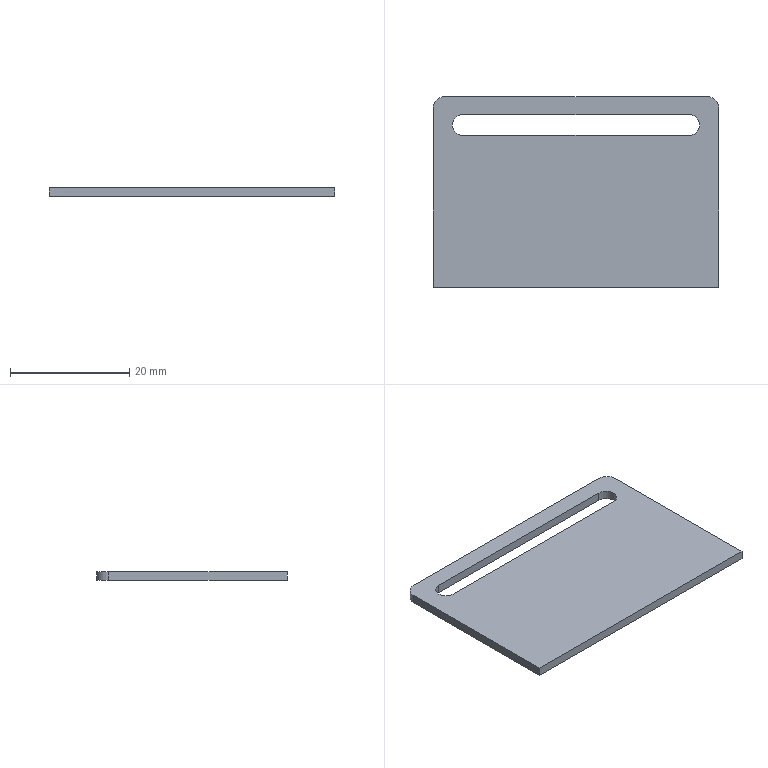Part | NX | features BREP 1 | 1 solid | 13 faces | box 48 x 32 x 1.5 mm | volume 2087 mm3 | plane 8 | cylinder 5 | commonest cylinder face diameters 3.5 x3 4 x2
STEP:
#1=CARTESIAN_POINT('',(24.,14.,1.5));
#2=VERTEX_POINT('',#1);
#3=CARTESIAN_POINT('',(22.,16.,1.5));
#4=VERTEX_POINT('',#3);
#5=CARTESIAN_POINT('',(22.,14.,1.5));
#6=DIRECTION('',(0.,0.,1.));
#7=DIRECTION('',(-1.,0.,0.));
#8=AXIS2_PLACEMENT_3D('',#5,#6,#7);
#9=CIRCLE('',#8,2.);
#10=EDGE_CURVE('',#2,#4,#9,.T.);
#11=ORIENTED_EDGE('',*,*,#10,.F.);
#12=CARTESIAN_POINT('',(24.,14.,0.));
#13=VERTEX_POINT('',#12);
#14=CARTESIAN_POINT('',(24.,14.,1.5));
#15=DIRECTION('',(0.,0.,1.));
#16=VECTOR('',#15,1000.);
#17=LINE('',#14,#16);
#18=EDGE_CURVE('',#13,#2,#17,.T.);
#19=ORIENTED_EDGE('',*,*,#18,.F.);
#20=CARTESIAN_POINT('',(22.,16.,0.));
#21=VERTEX_POINT('',#20);
#22=CARTESIAN_POINT('',(22.,14.,0.));
#23=DIRECTION('',(0.,0.,-1.));
#24=DIRECTION('',(-1.,0.,0.));
#25=AXIS2_PLACEMENT_3D('',#22,#23,#24);
#26=CIRCLE('',#25,2.);
#27=EDGE_CURVE('',#21,#13,#26,.T.);
#28=ORIENTED_EDGE('',*,*,#27,.F.);
#29=CARTESIAN_POINT('',(22.,16.,1.5));
#30=DIRECTION('',(0.,0.,-1.));
#31=VECTOR('',#30,1000.);
#32=LINE('',#29,#31);
#33=EDGE_CURVE('',#4,#21,#32,.T.);
#34=ORIENTED_EDGE('',*,*,#33,.F.);
#35=EDGE_LOOP('',(#11,#19,#28,#34));
#36=FACE_BOUND('',#35,.T.);
#37=CARTESIAN_POINT('',(22.,14.,1.5));
#38=DIRECTION('',(0.,0.,-1.));
#39=DIRECTION('',(-1.,0.,0.));
#40=AXIS2_PLACEMENT_3D('',#37,#38,#39);
#41=CYLINDRICAL_SURFACE('',#40,2.);
#42=ADVANCED_FACE('',(#36),#41,.T.);
#43=CARTESIAN_POINT('',(-22.,16.,1.5));
#44=VERTEX_POINT('',#43);
#45=CARTESIAN_POINT('',(-24.,14.,1.5));
#46=VERTEX_POINT('',#45);
#47=CARTESIAN_POINT('',(-22.,14.,1.5));
#48=DIRECTION('',(0.,0.,1.));
#49=DIRECTION('',(-1.,0.,0.));
#50=AXIS2_PLACEMENT_3D('',#47,#48,#49);
#51=CIRCLE('',#50,2.);
#52=EDGE_CURVE('',#44,#46,#51,.T.);
#53=ORIENTED_EDGE('',*,*,#52,.F.);
#54=CARTESIAN_POINT('',(-22.,16.,0.));
#55=VERTEX_POINT('',#54);
#56=CARTESIAN_POINT('',(-22.,16.,1.5));
#57=DIRECTION('',(0.,0.,1.));
#58=VECTOR('',#57,1000.);
#59=LINE('',#56,#58);
#60=EDGE_CURVE('',#55,#44,#59,.T.);
#61=ORIENTED_EDGE('',*,*,#60,.F.);
#62=CARTESIAN_POINT('',(-24.,14.,0.));
#63=VERTEX_POINT('',#62);
#64=CARTESIAN_POINT('',(-22.,14.,0.));
#65=DIRECTION('',(0.,0.,-1.));
#66=DIRECTION('',(-1.,0.,0.));
#67=AXIS2_PLACEMENT_3D('',#64,#65,#66);
#68=CIRCLE('',#67,2.);
#69=EDGE_CURVE('',#63,#55,#68,.T.);
#70=ORIENTED_EDGE('',*,*,#69,.F.);
#71=CARTESIAN_POINT('',(-24.,14.,1.5));
#72=DIRECTION('',(0.,0.,-1.));
#73=VECTOR('',#72,1000.);
#74=LINE('',#71,#73);
#75=EDGE_CURVE('',#46,#63,#74,.T.);
#76=ORIENTED_EDGE('',*,*,#75,.F.);
#77=EDGE_LOOP('',(#53,#61,#70,#76));
#78=FACE_BOUND('',#77,.T.);
#79=CARTESIAN_POINT('',(-22.,14.,1.5));
#80=DIRECTION('',(0.,0.,-1.));
#81=DIRECTION('',(-1.,0.,0.));
#82=AXIS2_PLACEMENT_3D('',#79,#80,#81);
#83=CYLINDRICAL_SURFACE('',#82,2.);
#84=ADVANCED_FACE('',(#78),#83,.T.);
#85=CARTESIAN_POINT('',(19.,13.,0.));
#86=VERTEX_POINT('',#85);
#87=CARTESIAN_POINT('',(-19.,13.,0.));
#88=VERTEX_POINT('',#87);
#89=CARTESIAN_POINT('',(-19.,13.,0.));
#90=DIRECTION('',(-1.,0.,0.));
#91=VECTOR('',#90,1000.);
#92=LINE('',#89,#91);
#93=EDGE_CURVE('',#86,#88,#92,.T.);
#94=ORIENTED_EDGE('',*,*,#93,.F.);
#95=CARTESIAN_POINT('',(19.,13.,1.5));
#96=VERTEX_POINT('',#95);
#97=CARTESIAN_POINT('',(19.,13.,1.5));
#98=DIRECTION('',(0.,0.,-1.));
#99=VECTOR('',#98,1000.);
#100=LINE('',#97,#99);
#101=EDGE_CURVE('',#96,#86,#100,.T.);
#102=ORIENTED_EDGE('',*,*,#101,.F.);
#103=CARTESIAN_POINT('',(-19.,13.,1.5));
#104=VERTEX_POINT('',#103);
#105=CARTESIAN_POINT('',(-19.,13.,1.5));
#106=DIRECTION('',(-1.,0.,0.));
#107=VECTOR('',#106,1000.);
#108=LINE('',#105,#107);
#109=EDGE_CURVE('',#96,#104,#108,.T.);
#110=ORIENTED_EDGE('',*,*,#109,.T.);
#111=CARTESIAN_POINT('',(-19.,13.,1.5));
#112=DIRECTION('',(0.,0.,-1.));
#113=VECTOR('',#112,1000.);
#114=LINE('',#111,#113);
#115=EDGE_CURVE('',#104,#88,#114,.T.);
#116=ORIENTED_EDGE('',*,*,#115,.T.);
#117=EDGE_LOOP('',(#94,#102,#110,#116));
#118=FACE_BOUND('',#117,.T.);
#119=CARTESIAN_POINT('',(-19.,13.,1.5));
#120=DIRECTION('',(0.,-1.,0.));
#121=DIRECTION('',(0.,0.,-1.));
#122=AXIS2_PLACEMENT_3D('',#119,#120,#121);
#123=PLANE('',#122);
#124=ADVANCED_FACE('',(#118),#123,.T.);
#125=CARTESIAN_POINT('',(19.,9.5,0.));
#126=VERTEX_POINT('',#125);
#127=CARTESIAN_POINT('',(19.,11.25,0.));
#128=DIRECTION('',(0.,0.,1.));
#129=DIRECTION('',(1.,0.,0.));
#130=AXIS2_PLACEMENT_3D('',#127,#128,#129);
#131=CIRCLE('',#130,1.75);
#132=EDGE_CURVE('',#126,#86,#131,.T.);
#133=ORIENTED_EDGE('',*,*,#132,.F.);
#134=CARTESIAN_POINT('',(19.,9.5,1.5));
#135=VERTEX_POINT('',#134);
#136=CARTESIAN_POINT('',(19.,9.5,1.5));
#137=DIRECTION('',(0.,0.,-1.));
#138=VECTOR('',#137,1000.);
#139=LINE('',#136,#138);
#140=EDGE_CURVE('',#135,#126,#139,.T.);
#141=ORIENTED_EDGE('',*,*,#140,.F.);
#142=CARTESIAN_POINT('',(19.,11.25,1.5));
#143=DIRECTION('',(0.,0.,1.));
#144=DIRECTION('',(1.,0.,0.));
#145=AXIS2_PLACEMENT_3D('',#142,#143,#144);
#146=CIRCLE('',#145,1.75);
#147=EDGE_CURVE('',#135,#96,#146,.T.);
#148=ORIENTED_EDGE('',*,*,#147,.T.);
#149=ORIENTED_EDGE('',*,*,#101,.T.);
#150=EDGE_LOOP('',(#133,#141,#148,#149));
#151=FACE_BOUND('',#150,.T.);
#152=CARTESIAN_POINT('',(19.,11.25,1.5));
#153=DIRECTION('',(0.,0.,-1.));
#154=DIRECTION('',(-1.,0.,0.));
#155=AXIS2_PLACEMENT_3D('',#152,#153,#154);
#156=CYLINDRICAL_SURFACE('',#155,1.75);
#157=ADVANCED_FACE('',(#151),#156,.F.);
#158=CARTESIAN_POINT('',(-19.,9.5,0.));
#159=VERTEX_POINT('',#158);
#160=CARTESIAN_POINT('',(-19.,9.5,0.));
#161=DIRECTION('',(1.,0.,0.));
#162=VECTOR('',#161,1000.);
#163=LINE('',#160,#162);
#164=EDGE_CURVE('',#159,#126,#163,.T.);
#165=ORIENTED_EDGE('',*,*,#164,.F.);
#166=CARTESIAN_POINT('',(-19.,9.5,1.5));
#167=VERTEX_POINT('',#166);
#168=CARTESIAN_POINT('',(-19.,9.5,1.5));
#169=DIRECTION('',(0.,0.,-1.));
#170=VECTOR('',#169,1000.);
#171=LINE('',#168,#170);
#172=EDGE_CURVE('',#167,#159,#171,.T.);
#173=ORIENTED_EDGE('',*,*,#172,.F.);
#174=CARTESIAN_POINT('',(-19.,9.5,1.5));
#175=DIRECTION('',(1.,0.,0.));
#176=VECTOR('',#175,1000.);
#177=LINE('',#174,#176);
#178=EDGE_CURVE('',#167,#135,#177,.T.);
#179=ORIENTED_EDGE('',*,*,#178,.T.);
#180=ORIENTED_EDGE('',*,*,#140,.T.);
#181=EDGE_LOOP('',(#165,#173,#179,#180));
#182=FACE_BOUND('',#181,.T.);
#183=CARTESIAN_POINT('',(-19.,9.5,1.5));
#184=DIRECTION('',(0.,1.,0.));
#185=DIRECTION('',(0.,0.,1.));
#186=AXIS2_PLACEMENT_3D('',#183,#184,#185);
#187=PLANE('',#186);
#188=ADVANCED_FACE('',(#182),#187,.T.);
#189=CARTESIAN_POINT('',(-20.75,11.25,1.5));
#190=VERTEX_POINT('',#189);
#191=CARTESIAN_POINT('',(-20.75,11.25,0.));
#192=VERTEX_POINT('',#191);
#193=CARTESIAN_POINT('',(-20.75,11.25,1.5));
#194=DIRECTION('',(0.,0.,-1.));
#195=VECTOR('',#194,1000.);
#196=LINE('',#193,#195);
#197=EDGE_CURVE('',#190,#192,#196,.T.);
#198=ORIENTED_EDGE('',*,*,#197,.F.);
#199=CARTESIAN_POINT('',(-19.,11.25,1.5));
#200=DIRECTION('',(0.,0.,1.));
#201=DIRECTION('',(1.,0.,0.));
#202=AXIS2_PLACEMENT_3D('',#199,#200,#201);
#203=CIRCLE('',#202,1.75);
#204=EDGE_CURVE('',#190,#167,#203,.T.);
#205=ORIENTED_EDGE('',*,*,#204,.T.);
#206=ORIENTED_EDGE('',*,*,#172,.T.);
#207=CARTESIAN_POINT('',(-19.,11.25,0.));
#208=DIRECTION('',(0.,0.,1.));
#209=DIRECTION('',(1.,0.,0.));
#210=AXIS2_PLACEMENT_3D('',#207,#208,#209);
#211=CIRCLE('',#210,1.75);
#212=EDGE_CURVE('',#192,#159,#211,.T.);
#213=ORIENTED_EDGE('',*,*,#212,.F.);
#214=EDGE_LOOP('',(#198,#205,#206,#213));
#215=FACE_BOUND('',#214,.T.);
#216=CARTESIAN_POINT('',(-19.,11.25,1.5));
#217=DIRECTION('',(0.,0.,-1.));
#218=DIRECTION('',(-1.,0.,0.));
#219=AXIS2_PLACEMENT_3D('',#216,#217,#218);
#220=CYLINDRICAL_SURFACE('',#219,1.75);
#221=ADVANCED_FACE('',(#215),#220,.F.);
#222=CARTESIAN_POINT('',(-24.,-16.,0.));
#223=VERTEX_POINT('',#222);
#224=CARTESIAN_POINT('',(24.,-16.,0.));
#225=VERTEX_POINT('',#224);
#226=CARTESIAN_POINT('',(-24.,-16.,0.));
#227=DIRECTION('',(1.,0.,0.));
#228=VECTOR('',#227,1000.);
#229=LINE('',#226,#228);
#230=EDGE_CURVE('',#223,#225,#229,.T.);
#231=ORIENTED_EDGE('',*,*,#230,.T.);
#232=CARTESIAN_POINT('',(24.,-16.,1.5));
#233=VERTEX_POINT('',#232);
#234=CARTESIAN_POINT('',(24.,-16.,1.5));
#235=DIRECTION('',(0.,0.,-1.));
#236=VECTOR('',#235,1000.);
#237=LINE('',#234,#236);
#238=EDGE_CURVE('',#233,#225,#237,.T.);
#239=ORIENTED_EDGE('',*,*,#238,.F.);
#240=CARTESIAN_POINT('',(-24.,-16.,1.5));
#241=VERTEX_POINT('',#240);
#242=CARTESIAN_POINT('',(-24.,-16.,1.5));
#243=DIRECTION('',(1.,0.,0.));
#244=VECTOR('',#243,1000.);
#245=LINE('',#242,#244);
#246=EDGE_CURVE('',#241,#233,#245,.T.);
#247=ORIENTED_EDGE('',*,*,#246,.F.);
#248=CARTESIAN_POINT('',(-24.,-16.,1.5));
#249=DIRECTION('',(0.,0.,-1.));
#250=VECTOR('',#249,1000.);
#251=LINE('',#248,#250);
#252=EDGE_CURVE('',#241,#223,#251,.T.);
#253=ORIENTED_EDGE('',*,*,#252,.T.);
#254=EDGE_LOOP('',(#231,#239,#247,#253));
#255=FACE_BOUND('',#254,.T.);
#256=CARTESIAN_POINT('',(-24.,-16.,1.5));
#257=DIRECTION('',(0.,1.,0.));
#258=DIRECTION('',(0.,0.,1.));
#259=AXIS2_PLACEMENT_3D('',#256,#257,#258);
#260=PLANE('',#259);
#261=ADVANCED_FACE('',(#255),#260,.F.);
#262=CARTESIAN_POINT('',(-24.,-16.,1.5));
#263=DIRECTION('',(0.,-1.,0.));
#264=VECTOR('',#263,1000.);
#265=LINE('',#262,#264);
#266=EDGE_CURVE('',#46,#241,#265,.T.);
#267=ORIENTED_EDGE('',*,*,#266,.F.);
#268=ORIENTED_EDGE('',*,*,#75,.T.);
#269=CARTESIAN_POINT('',(-24.,-16.,0.));
#270=DIRECTION('',(0.,-1.,0.));
#271=VECTOR('',#270,1000.);
#272=LINE('',#269,#271);
#273=EDGE_CURVE('',#63,#223,#272,.T.);
#274=ORIENTED_EDGE('',*,*,#273,.T.);
#275=ORIENTED_EDGE('',*,*,#252,.F.);
#276=EDGE_LOOP('',(#267,#268,#274,#275));
#277=FACE_BOUND('',#276,.T.);
#278=CARTESIAN_POINT('',(-24.,-16.,1.5));
#279=DIRECTION('',(1.,0.,0.));
#280=DIRECTION('',(0.,0.,-1.));
#281=AXIS2_PLACEMENT_3D('',#278,#279,#280);
#282=PLANE('',#281);
#283=ADVANCED_FACE('',(#277),#282,.F.);
#284=CARTESIAN_POINT('',(-24.,16.,0.));
#285=DIRECTION('',(-1.,0.,0.));
#286=VECTOR('',#285,1000.);
#287=LINE('',#284,#286);
#288=EDGE_CURVE('',#21,#55,#287,.T.);
#289=ORIENTED_EDGE('',*,*,#288,.T.);
#290=ORIENTED_EDGE('',*,*,#60,.T.);
#291=CARTESIAN_POINT('',(-24.,16.,1.5));
#292=DIRECTION('',(-1.,0.,0.));
#293=VECTOR('',#292,1000.);
#294=LINE('',#291,#293);
#295=EDGE_CURVE('',#4,#44,#294,.T.);
#296=ORIENTED_EDGE('',*,*,#295,.F.);
#297=ORIENTED_EDGE('',*,*,#33,.T.);
#298=EDGE_LOOP('',(#289,#290,#296,#297));
#299=FACE_BOUND('',#298,.T.);
#300=CARTESIAN_POINT('',(-24.,16.,1.5));
#301=DIRECTION('',(0.,-1.,0.));
#302=DIRECTION('',(0.,0.,-1.));
#303=AXIS2_PLACEMENT_3D('',#300,#301,#302);
#304=PLANE('',#303);
#305=ADVANCED_FACE('',(#299),#304,.F.);
#306=CARTESIAN_POINT('',(24.,-16.,0.));
#307=DIRECTION('',(0.,1.,0.));
#308=VECTOR('',#307,1000.);
#309=LINE('',#306,#308);
#310=EDGE_CURVE('',#225,#13,#309,.T.);
#311=ORIENTED_EDGE('',*,*,#310,.T.);
#312=ORIENTED_EDGE('',*,*,#18,.T.);
#313=CARTESIAN_POINT('',(24.,-16.,1.5));
#314=DIRECTION('',(0.,1.,0.));
#315=VECTOR('',#314,1000.);
#316=LINE('',#313,#315);
#317=EDGE_CURVE('',#233,#2,#316,.T.);
#318=ORIENTED_EDGE('',*,*,#317,.F.);
#319=ORIENTED_EDGE('',*,*,#238,.T.);
#320=EDGE_LOOP('',(#311,#312,#318,#319));
#321=FACE_BOUND('',#320,.T.);
#322=CARTESIAN_POINT('',(24.,-16.,1.5));
#323=DIRECTION('',(-1.,0.,0.));
#324=DIRECTION('',(0.,0.,1.));
#325=AXIS2_PLACEMENT_3D('',#322,#323,#324);
#326=PLANE('',#325);
#327=ADVANCED_FACE('',(#321),#326,.F.);
#328=ORIENTED_EDGE('',*,*,#93,.T.);
#329=CARTESIAN_POINT('',(-19.,11.25,0.));
#330=DIRECTION('',(0.,0.,1.));
#331=DIRECTION('',(1.,0.,0.));
#332=AXIS2_PLACEMENT_3D('',#329,#330,#331);
#333=CIRCLE('',#332,1.75);
#334=EDGE_CURVE('',#88,#192,#333,.T.);
#335=ORIENTED_EDGE('',*,*,#334,.T.);
#336=ORIENTED_EDGE('',*,*,#212,.T.);
#337=ORIENTED_EDGE('',*,*,#164,.T.);
#338=ORIENTED_EDGE('',*,*,#132,.T.);
#339=EDGE_LOOP('',(#328,#335,#336,#337,#338));
#340=FACE_BOUND('',#339,.T.);
#341=ORIENTED_EDGE('',*,*,#273,.F.);
#342=ORIENTED_EDGE('',*,*,#69,.T.);
#343=ORIENTED_EDGE('',*,*,#288,.F.);
#344=ORIENTED_EDGE('',*,*,#27,.T.);
#345=ORIENTED_EDGE('',*,*,#310,.F.);
#346=ORIENTED_EDGE('',*,*,#230,.F.);
#347=EDGE_LOOP('',(#341,#342,#343,#344,#345,#346));
#348=FACE_BOUND('',#347,.T.);
#349=CARTESIAN_POINT('',(0.,0.,0.));
#350=DIRECTION('',(0.,0.,-1.));
#351=DIRECTION('',(-1.,0.,0.));
#352=AXIS2_PLACEMENT_3D('',#349,#350,#351);
#353=PLANE('',#352);
#354=ADVANCED_FACE('',(#340,#348),#353,.T.);
#355=CARTESIAN_POINT('',(-19.,11.25,1.5));
#356=DIRECTION('',(0.,0.,1.));
#357=DIRECTION('',(1.,0.,0.));
#358=AXIS2_PLACEMENT_3D('',#355,#356,#357);
#359=CIRCLE('',#358,1.75);
#360=EDGE_CURVE('',#104,#190,#359,.T.);
#361=ORIENTED_EDGE('',*,*,#360,.F.);
#362=ORIENTED_EDGE('',*,*,#109,.F.);
#363=ORIENTED_EDGE('',*,*,#147,.F.);
#364=ORIENTED_EDGE('',*,*,#178,.F.);
#365=ORIENTED_EDGE('',*,*,#204,.F.);
#366=EDGE_LOOP('',(#361,#362,#363,#364,#365));
#367=FACE_BOUND('',#366,.T.);
#368=ORIENTED_EDGE('',*,*,#295,.T.);
#369=ORIENTED_EDGE('',*,*,#52,.T.);
#370=ORIENTED_EDGE('',*,*,#266,.T.);
#371=ORIENTED_EDGE('',*,*,#246,.T.);
#372=ORIENTED_EDGE('',*,*,#317,.T.);
#373=ORIENTED_EDGE('',*,*,#10,.T.);
#374=EDGE_LOOP('',(#368,#369,#370,#371,#372,#373));
#375=FACE_BOUND('',#374,.T.);
#376=CARTESIAN_POINT('',(0.,0.,1.5));
#377=DIRECTION('',(0.,0.,-1.));
#378=DIRECTION('',(-1.,0.,0.));
#379=AXIS2_PLACEMENT_3D('',#376,#377,#378);
#380=PLANE('',#379);
#381=ADVANCED_FACE('',(#367,#375),#380,.F.);
#382=ORIENTED_EDGE('',*,*,#360,.T.);
#383=ORIENTED_EDGE('',*,*,#197,.T.);
#384=ORIENTED_EDGE('',*,*,#334,.F.);
#385=ORIENTED_EDGE('',*,*,#115,.F.);
#386=EDGE_LOOP('',(#382,#383,#384,#385));
#387=FACE_BOUND('',#386,.T.);
#388=CARTESIAN_POINT('',(-19.,11.25,1.5));
#389=DIRECTION('',(0.,0.,-1.));
#390=DIRECTION('',(-1.,0.,0.));
#391=AXIS2_PLACEMENT_3D('',#388,#389,#390);
#392=CYLINDRICAL_SURFACE('',#391,1.75);
#393=ADVANCED_FACE('',(#387),#392,.F.);
#394=CLOSED_SHELL('',(#42,#84,#124,#157,#188,#221,#261,#283,#305,#327,#354,#381,#393));
#395=MANIFOLD_SOLID_BREP('',#394);
#396=(LENGTH_UNIT()NAMED_UNIT(*)SI_UNIT(.MILLI.,.METRE.));
#397=UNCERTAINTY_MEASURE_WITH_UNIT(LENGTH_MEASURE(0.00001),#396,'','');
#398=(NAMED_UNIT(*)PLANE_ANGLE_UNIT()SI_UNIT($,.RADIAN.));
#399=(NAMED_UNIT(*)SI_UNIT($,.STERADIAN.)SOLID_ANGLE_UNIT());
#400=(GEOMETRIC_REPRESENTATION_CONTEXT(3)GLOBAL_UNCERTAINTY_ASSIGNED_CONTEXT((#397))GLOBAL_UNIT_ASSIGNED_CONTEXT((#396,#398,#399))REPRESENTATION_CONTEXT('',''));
#401=ADVANCED_BREP_SHAPE_REPRESENTATION('',(#395),#400);